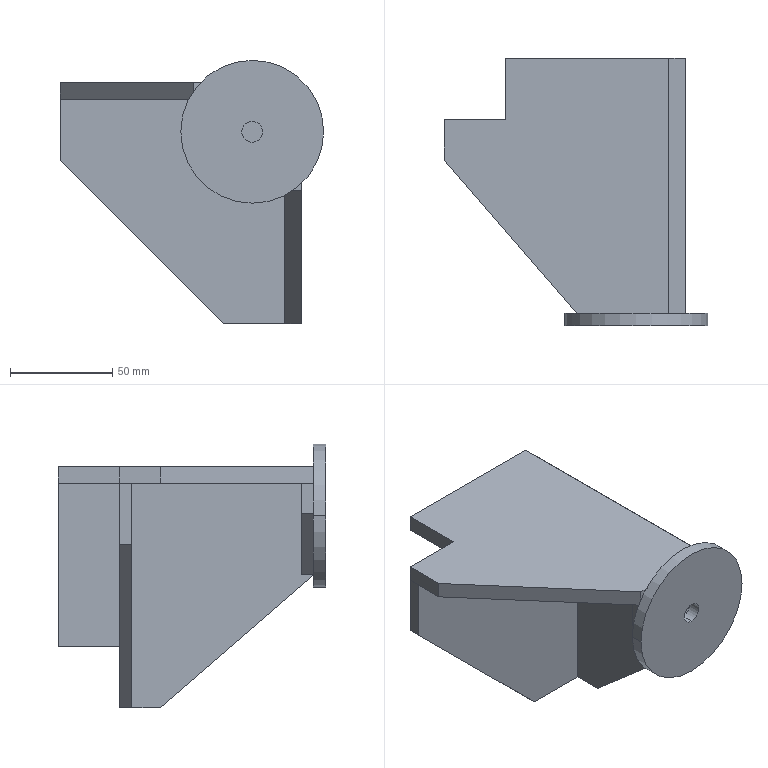Part | STEP file | Foot support 01001 | 5 solids | 42 faces | box 129 x 131 x 129 mm | volume 250060 mm3 | plane 36 | cylinder 6 | commonest cylinder face diameters 10.2 x4 70 x2